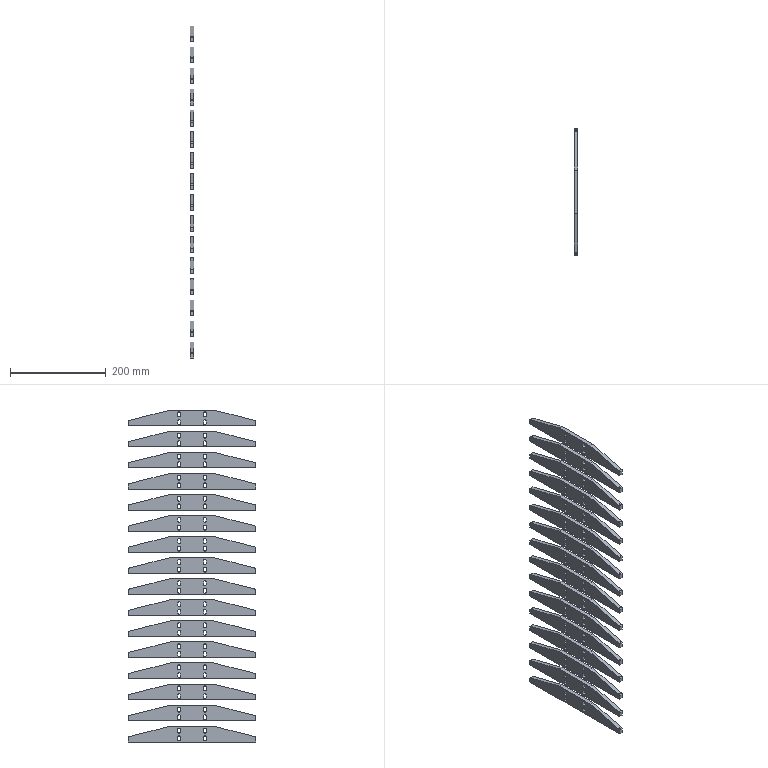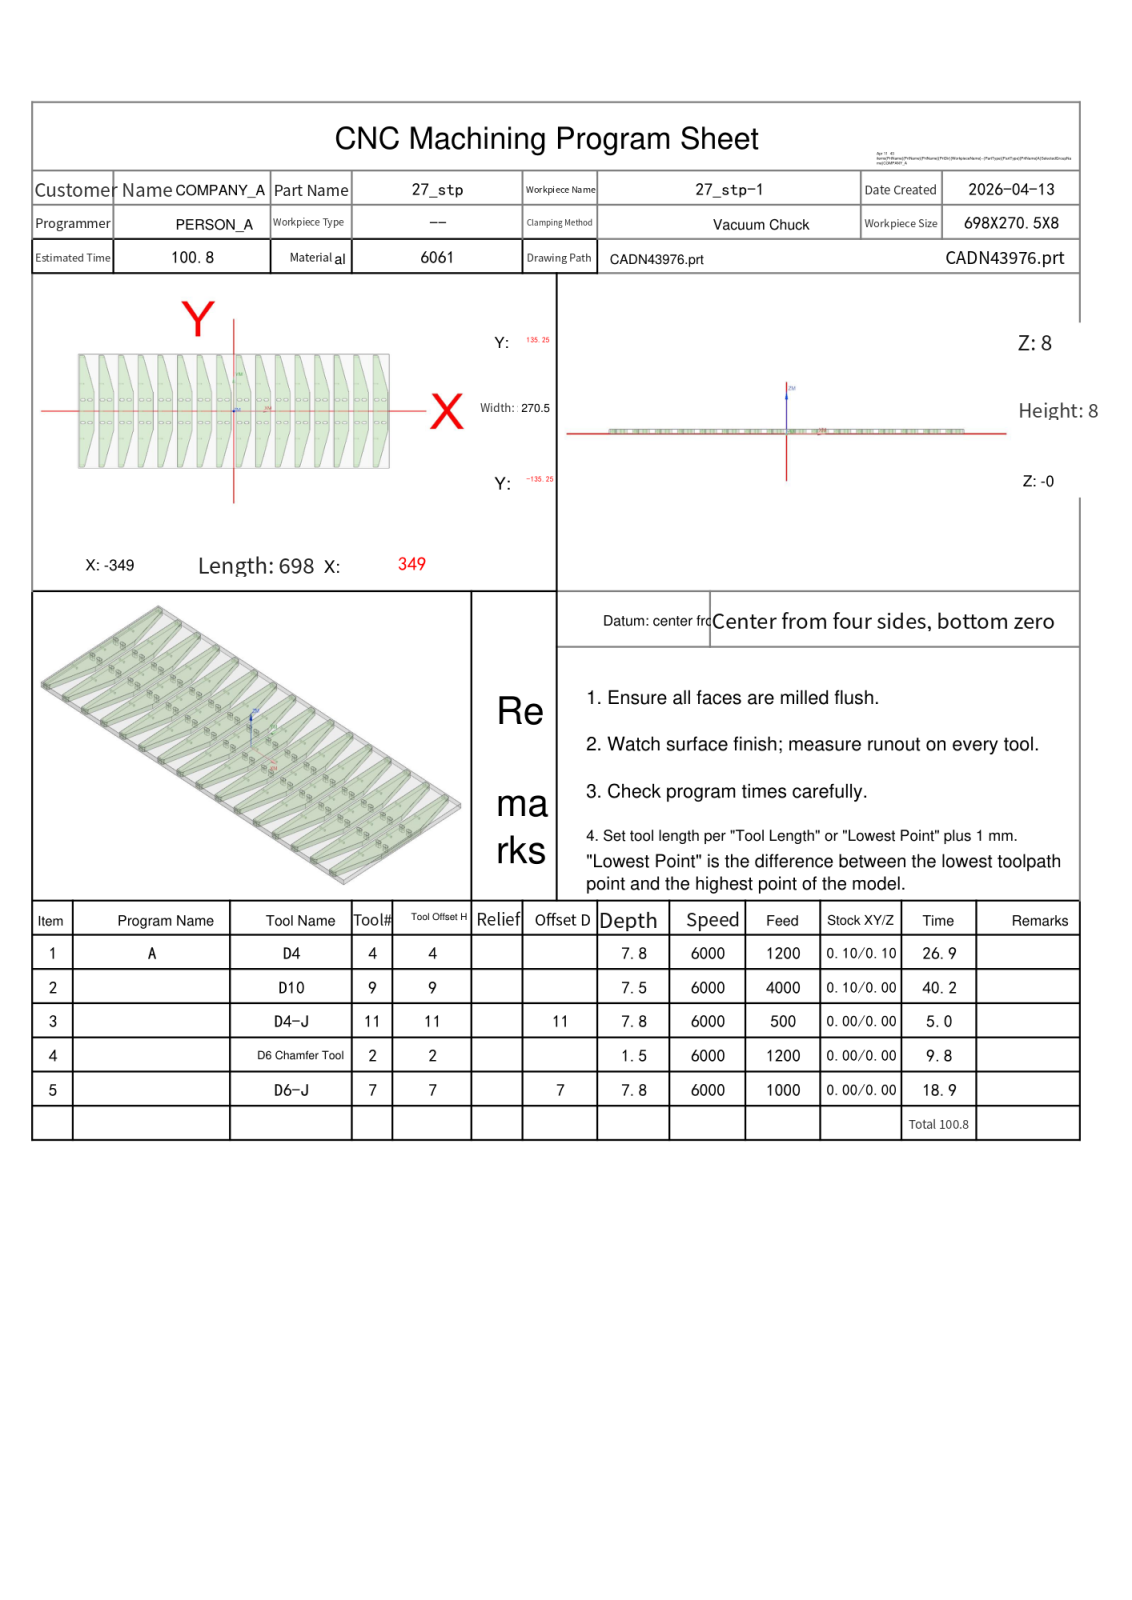NC program | NX | posted by the shop | part box 8 x 265.5 x 693 mm
Lines 14218 to 15115 of 21683:
N2 T09 M06
(D10  D=10. R=0. H=09 ce=0.10 di=0.00)
G00 G90 G54 X307.6 Y0.0 M03 S6000
G43 H09 Z28.
M08
Z8.5
G01 Y-45.801 Z8.461 F4000.
X285.864 Y-131.736 Z8.386
G02 X278.012 Y-137.85 Z8.377 I-7.853 J1.986
G01 X269.5 Z8.37
G02 X264.4 Y-132.75 Z8.363 I0.0 J5.1
G01 Y132.75 Z8.137
G02 X269.5 Y137.85 Z8.13 I5.1 J0.0
G01 X278.012 Z8.123
G02 X285.864 Y131.736 Z8.114 I0.0 J-8.1
G01 X307.6 Y45.801 Z8.039
Y-45.801 Z7.961
X285.864 Y-131.736 Z7.886
G02 X278.012 Y-137.85 Z7.877 I-7.853 J1.986
G01 X269.5 Z7.87
G02 X264.4 Y-132.75 Z7.863 I0.0 J5.1
G01 Y132.75 Z7.637
G02 X269.5 Y137.85 Z7.63 I5.1 J0.0
G01 X278.012 Z7.623
G02 X285.864 Y131.736 Z7.614 I0.0 J-8.1
G01 X307.6 Y45.801 Z7.539
Y-45.801 Z7.461
X285.864 Y-131.736 Z7.386
G02 X278.012 Y-137.85 Z7.377 I-7.853 J1.986
G01 X269.5 Z7.37
G02 X264.4 Y-132.75 Z7.363 I0.0 J5.1
G01 Y132.75 Z7.137
G02 X269.5 Y137.85 Z7.13 I5.1 J0.0
G01 X278.012 Z7.123
G02 X285.864 Y131.736 Z7.114 I0.0 J-8.1
G01 X307.6 Y45.801 Z7.039
Y-45.801 Z6.961
X285.864 Y-131.736 Z6.886
G02 X278.012 Y-137.85 Z6.877 I-7.853 J1.986
G01 X269.5 Z6.87
G02 X264.4 Y-132.75 Z6.863 I0.0 J5.1
G01 Y132.75 Z6.637
G02 X269.5 Y137.85 Z6.63 I5.1 J0.0
G01 X278.012 Z6.623
G02 X285.864 Y131.736 Z6.614 I0.0 J-8.1
G01 X307.6 Y45.801 Z6.539
Y-45.801 Z6.461
X285.864 Y-131.736 Z6.386
G02 X278.012 Y-137.85 Z6.377 I-7.853 J1.986
G01 X269.5 Z6.37
G02 X264.4 Y-132.75 Z6.363 I0.0 J5.1
G01 Y132.75 Z6.137
G02 X269.5 Y137.85 Z6.13 I5.1 J0.0
G01 X278.012 Z6.123
G02 X285.864 Y131.736 Z6.114 I0.0 J-8.1
G01 X307.6 Y45.801 Z6.039
Y-45.801 Z5.961
X285.864 Y-131.736 Z5.886
G02 X278.012 Y-137.85 Z5.877 I-7.853 J1.986
G01 X269.5 Z5.87
G02 X264.4 Y-132.75 Z5.863 I0.0 J5.1
G01 Y132.75 Z5.637
G02 X269.5 Y137.85 Z5.63 I5.1 J0.0
G01 X278.012 Z5.623
G02 X285.864 Y131.736 Z5.614 I0.0 J-8.1
G01 X307.6 Y45.801 Z5.539
Y-45.801 Z5.461
X285.864 Y-131.736 Z5.386
G02 X278.012 Y-137.85 Z5.377 I-7.853 J1.986
G01 X269.5 Z5.37
G02 X264.4 Y-132.75 Z5.363 I0.0 J5.1
G01 Y132.75 Z5.137
G02 X269.5 Y137.85 Z5.13 I5.1 J0.0
G01 X278.012 Z5.123
G02 X285.864 Y131.736 Z5.114 I0.0 J-8.1
G01 X307.6 Y45.801 Z5.039
Y-45.801 Z4.961
X285.864 Y-131.736 Z4.886
G02 X278.012 Y-137.85 Z4.877 I-7.853 J1.986
G01 X269.5 Z4.87
G02 X264.4 Y-132.75 Z4.863 I0.0 J5.1
G01 Y132.75 Z4.637
G02 X269.5 Y137.85 Z4.63 I5.1 J0.0
G01 X278.012 Z4.623
G02 X285.864 Y131.736 Z4.614 I0.0 J-8.1
G01 X307.6 Y45.801 Z4.539
Y-45.801 Z4.461
X285.864 Y-131.736 Z4.386
G02 X278.012 Y-137.85 Z4.377 I-7.853 J1.986
G01 X269.5 Z4.37
G02 X264.4 Y-132.75 Z4.363 I0.0 J5.1
G01 Y132.75 Z4.137
G02 X269.5 Y137.85 Z4.13 I5.1 J0.0
G01 X278.012 Z4.123
G02 X285.864 Y131.736 Z4.114 I0.0 J-8.1
G01 X307.6 Y45.801 Z4.039
Y-45.801 Z3.961
X285.864 Y-131.736 Z3.886
G02 X278.012 Y-137.85 Z3.877 I-7.853 J1.986
G01 X269.5 Z3.87
G02 X264.4 Y-132.75 Z3.863 I0.0 J5.1
G01 Y132.75 Z3.637
G02 X269.5 Y137.85 Z3.63 I5.1 J0.0
G01 X278.012 Z3.623
G02 X285.864 Y131.736 Z3.614 I0.0 J-8.1
G01 X307.6 Y45.801 Z3.539
Y-45.801 Z3.461
X285.864 Y-131.736 Z3.386
G02 X278.012 Y-137.85 Z3.377 I-7.853 J1.986
G01 X269.5 Z3.37
G02 X264.4 Y-132.75 Z3.363 I0.0 J5.1
G01 Y132.75 Z3.137
G02 X269.5 Y137.85 Z3.13 I5.1 J0.0
G01 X278.012 Z3.123
G02 X285.864 Y131.736 Z3.114 I0.0 J-8.1
G01 X307.6 Y45.801 Z3.039
Y-45.801 Z2.961
X285.864 Y-131.736 Z2.886
G02 X278.012 Y-137.85 Z2.877 I-7.853 J1.986
G01 X269.5 Z2.87
G02 X264.4 Y-132.75 Z2.863 I0.0 J5.1
G01 Y132.75 Z2.637
G02 X269.5 Y137.85 Z2.63 I5.1 J0.0
G01 X278.012 Z2.623
G02 X285.864 Y131.736 Z2.614 I0.0 J-8.1
G01 X307.6 Y45.801 Z2.539
Y-45.801 Z2.461
X285.864 Y-131.736 Z2.386
G02 X278.012 Y-137.85 Z2.377 I-7.853 J1.986
G01 X269.5 Z2.37
G02 X264.4 Y-132.75 Z2.363 I0.0 J5.1
G01 Y132.75 Z2.137
G02 X269.5 Y137.85 Z2.13 I5.1 J0.0
G01 X278.012 Z2.123
G02 X285.864 Y131.736 Z2.114 I0.0 J-8.1
G01 X307.6 Y45.801 Z2.039
Y-45.801 Z1.961
X285.864 Y-131.736 Z1.886
G02 X278.012 Y-137.85 Z1.877 I-7.853 J1.986
G01 X269.5 Z1.87
G02 X264.4 Y-132.75 Z1.863 I0.0 J5.1
G01 Y132.75 Z1.637
G02 X269.5 Y137.85 Z1.63 I5.1 J0.0
G01 X278.012 Z1.623
G02 X285.864 Y131.736 Z1.614 I0.0 J-8.1
G01 X307.6 Y45.801 Z1.539
Y-45.801 Z1.461
X285.864 Y-131.736 Z1.386
G02 X278.012 Y-137.85 Z1.377 I-7.853 J1.986
G01 X269.5 Z1.37
G02 X264.4 Y-132.75 Z1.363 I0.0 J5.1
G01 Y132.75 Z1.137
G02 X269.5 Y137.85 Z1.13 I5.1 J0.0
G01 X278.012 Z1.123
G02 X285.864 Y131.736 Z1.114 I0.0 J-8.1
G01 X307.6 Y45.801 Z1.039
Y-45.801 Z.961
X285.864 Y-131.736 Z.886
G02 X278.012 Y-137.85 Z.877 I-7.853 J1.986
G01 X269.5 Z.87
G02 X264.4 Y-132.75 Z.863 I0.0 J5.1
G01 Y132.75 Z.637
G02 X269.5 Y137.85 Z.63 I5.1 J0.0
G01 X278.012 Z.623
G02 X285.864 Y131.736 Z.614 I0.0 J-8.1
G01 X307.6 Y45.801 Z.539
Y0.0 Z.5
Y-45.801
X285.864 Y-131.736
G02 X278.012 Y-137.85 I-7.853 J1.986
G01 X269.5
G02 X264.4 Y-132.75 I0.0 J5.1
G01 Y132.75
G02 X269.5 Y137.85 I5.1 J0.0
G01 X278.012
G02 X285.864 Y131.736 I0.0 J-8.1
G01 X307.6 Y45.801
Y0.0
Y-.5
Z1.5
G00 Z28.
X351.6 Y0.0
Z8.5
G01 Y-45.801 Z8.461
X329.864 Y-131.736 Z8.386
G02 X322.012 Y-137.85 Z8.377 I-7.853 J1.986
G01 X313.5 Z8.37
G02 X308.4 Y-132.75 Z8.363 I0.0 J5.1
G01 Y132.75 Z8.137
G02 X313.5 Y137.85 Z8.13 I5.1 J0.0
G01 X322.012 Z8.123
G02 X329.864 Y131.736 Z8.114 I0.0 J-8.1
G01 X351.6 Y45.801 Z8.039
Y-45.801 Z7.961
X329.864 Y-131.736 Z7.886
G02 X322.012 Y-137.85 Z7.877 I-7.853 J1.986
G01 X313.5 Z7.87
G02 X308.4 Y-132.75 Z7.863 I0.0 J5.1
G01 Y132.75 Z7.637
G02 X313.5 Y137.85 Z7.63 I5.1 J0.0
G01 X322.012 Z7.623
G02 X329.864 Y131.736 Z7.614 I0.0 J-8.1
G01 X351.6 Y45.801 Z7.539
Y-45.801 Z7.461
X329.864 Y-131.736 Z7.386
G02 X322.012 Y-137.85 Z7.377 I-7.853 J1.986
G01 X313.5 Z7.37
G02 X308.4 Y-132.75 Z7.363 I0.0 J5.1
G01 Y132.75 Z7.137
G02 X313.5 Y137.85 Z7.13 I5.1 J0.0
G01 X322.012 Z7.123
G02 X329.864 Y131.736 Z7.114 I0.0 J-8.1
G01 X351.6 Y45.801 Z7.039
Y-45.801 Z6.961
X329.864 Y-131.736 Z6.886
G02 X322.012 Y-137.85 Z6.877 I-7.853 J1.986
G01 X313.5 Z6.87
G02 X308.4 Y-132.75 Z6.863 I0.0 J5.1
G01 Y132.75 Z6.637
G02 X313.5 Y137.85 Z6.63 I5.1 J0.0
G01 X322.012 Z6.623
G02 X329.864 Y131.736 Z6.614 I0.0 J-8.1
G01 X351.6 Y45.801 Z6.539
Y-45.801 Z6.461
X329.864 Y-131.736 Z6.386
G02 X322.012 Y-137.85 Z6.377 I-7.853 J1.986
G01 X313.5 Z6.37
G02 X308.4 Y-132.75 Z6.363 I0.0 J5.1
G01 Y132.75 Z6.137
G02 X313.5 Y137.85 Z6.13 I5.1 J0.0
G01 X322.012 Z6.123
G02 X329.864 Y131.736 Z6.114 I0.0 J-8.1
G01 X351.6 Y45.801 Z6.039
Y-45.801 Z5.961
X329.864 Y-131.736 Z5.886
G02 X322.012 Y-137.85 Z5.877 I-7.853 J1.986
G01 X313.5 Z5.87
G02 X308.4 Y-132.75 Z5.863 I0.0 J5.1
G01 Y132.75 Z5.637
G02 X313.5 Y137.85 Z5.63 I5.1 J0.0
G01 X322.012 Z5.623
G02 X329.864 Y131.736 Z5.614 I0.0 J-8.1
G01 X351.6 Y45.801 Z5.539
Y-45.801 Z5.461
X329.864 Y-131.736 Z5.386
G02 X322.012 Y-137.85 Z5.377 I-7.853 J1.986
G01 X313.5 Z5.37
G02 X308.4 Y-132.75 Z5.363 I0.0 J5.1
G01 Y132.75 Z5.137
G02 X313.5 Y137.85 Z5.13 I5.1 J0.0
G01 X322.012 Z5.123
G02 X329.864 Y131.736 Z5.114 I0.0 J-8.1
G01 X351.6 Y45.801 Z5.039
Y-45.801 Z4.961
X329.864 Y-131.736 Z4.886
G02 X322.012 Y-137.85 Z4.877 I-7.853 J1.986
G01 X313.5 Z4.87
G02 X308.4 Y-132.75 Z4.863 I0.0 J5.1
G01 Y132.75 Z4.637
G02 X313.5 Y137.85 Z4.63 I5.1 J0.0
G01 X322.012 Z4.623
G02 X329.864 Y131.736 Z4.614 I0.0 J-8.1
G01 X351.6 Y45.801 Z4.539
Y-45.801 Z4.461
X329.864 Y-131.736 Z4.386
G02 X322.012 Y-137.85 Z4.377 I-7.853 J1.986
G01 X313.5 Z4.37
G02 X308.4 Y-132.75 Z4.363 I0.0 J5.1
G01 Y132.75 Z4.137
G02 X313.5 Y137.85 Z4.13 I5.1 J0.0
G01 X322.012 Z4.123
G02 X329.864 Y131.736 Z4.114 I0.0 J-8.1
G01 X351.6 Y45.801 Z4.039
Y-45.801 Z3.961
X329.864 Y-131.736 Z3.886
G02 X322.012 Y-137.85 Z3.877 I-7.853 J1.986
G01 X313.5 Z3.87
G02 X308.4 Y-132.75 Z3.863 I0.0 J5.1
G01 Y132.75 Z3.637
G02 X313.5 Y137.85 Z3.63 I5.1 J0.0
G01 X322.012 Z3.623
G02 X329.864 Y131.736 Z3.614 I0.0 J-8.1
G01 X351.6 Y45.801 Z3.539
Y-45.801 Z3.461
X329.864 Y-131.736 Z3.386
G02 X322.012 Y-137.85 Z3.377 I-7.853 J1.986
G01 X313.5 Z3.37
G02 X308.4 Y-132.75 Z3.363 I0.0 J5.1
G01 Y132.75 Z3.137
G02 X313.5 Y137.85 Z3.13 I5.1 J0.0
G01 X322.012 Z3.123
G02 X329.864 Y131.736 Z3.114 I0.0 J-8.1
G01 X351.6 Y45.801 Z3.039
Y-45.801 Z2.961
X329.864 Y-131.736 Z2.886
G02 X322.012 Y-137.85 Z2.877 I-7.853 J1.986
G01 X313.5 Z2.87
G02 X308.4 Y-132.75 Z2.863 I0.0 J5.1
G01 Y132.75 Z2.637
G02 X313.5 Y137.85 Z2.63 I5.1 J0.0
G01 X322.012 Z2.623
G02 X329.864 Y131.736 Z2.614 I0.0 J-8.1
G01 X351.6 Y45.801 Z2.539
Y-45.801 Z2.461
X329.864 Y-131.736 Z2.386
G02 X322.012 Y-137.85 Z2.377 I-7.853 J1.986
G01 X313.5 Z2.37
G02 X308.4 Y-132.75 Z2.363 I0.0 J5.1
G01 Y132.75 Z2.137
G02 X313.5 Y137.85 Z2.13 I5.1 J0.0
G01 X322.012 Z2.123
G02 X329.864 Y131.736 Z2.114 I0.0 J-8.1
G01 X351.6 Y45.801 Z2.039
Y-45.801 Z1.961
X329.864 Y-131.736 Z1.886
G02 X322.012 Y-137.85 Z1.877 I-7.853 J1.986
G01 X313.5 Z1.87
G02 X308.4 Y-132.75 Z1.863 I0.0 J5.1
G01 Y132.75 Z1.637
G02 X313.5 Y137.85 Z1.63 I5.1 J0.0
G01 X322.012 Z1.623
G02 X329.864 Y131.736 Z1.614 I0.0 J-8.1
G01 X351.6 Y45.801 Z1.539
Y-45.801 Z1.461
X329.864 Y-131.736 Z1.386
G02 X322.012 Y-137.85 Z1.377 I-7.853 J1.986
G01 X313.5 Z1.37
G02 X308.4 Y-132.75 Z1.363 I0.0 J5.1
G01 Y132.75 Z1.137
G02 X313.5 Y137.85 Z1.13 I5.1 J0.0
G01 X322.012 Z1.123
G02 X329.864 Y131.736 Z1.114 I0.0 J-8.1
G01 X351.6 Y45.801 Z1.039
Y-45.801 Z.961
X329.864 Y-131.736 Z.886
G02 X322.012 Y-137.85 Z.877 I-7.853 J1.986
G01 X313.5 Z.87
G02 X308.4 Y-132.75 Z.863 I0.0 J5.1
G01 Y132.75 Z.637
G02 X313.5 Y137.85 Z.63 I5.1 J0.0
G01 X322.012 Z.623
G02 X329.864 Y131.736 Z.614 I0.0 J-8.1
G01 X351.6 Y45.801 Z.539
Y0.0 Z.5
Y-45.801
X329.864 Y-131.736
G02 X322.012 Y-137.85 I-7.853 J1.986
G01 X313.5
G02 X308.4 Y-132.75 I0.0 J5.1
G01 Y132.75
G02 X313.5 Y137.85 I5.1 J0.0
G01 X322.012
G02 X329.864 Y131.736 I0.0 J-8.1
G01 X351.6 Y45.801
Y0.0
Y-.5
Z1.5
G00 Z28.
X263.6 Y0.0
Z8.5
G01 Y-45.801 Z8.461
X241.864 Y-131.736 Z8.386
G02 X234.012 Y-137.85 Z8.377 I-7.853 J1.986
G01 X225.5 Z8.37
G02 X220.4 Y-132.75 Z8.363 I0.0 J5.1
G01 Y132.75 Z8.137
G02 X225.5 Y137.85 Z8.13 I5.1 J0.0
G01 X234.012 Z8.123
G02 X241.864 Y131.736 Z8.114 I0.0 J-8.1
G01 X263.6 Y45.801 Z8.039
Y-45.801 Z7.961
X241.864 Y-131.736 Z7.886
G02 X234.012 Y-137.85 Z7.877 I-7.853 J1.986
G01 X225.5 Z7.87
G02 X220.4 Y-132.75 Z7.863 I0.0 J5.1
G01 Y132.75 Z7.637
G02 X225.5 Y137.85 Z7.63 I5.1 J0.0
G01 X234.012 Z7.623
G02 X241.864 Y131.736 Z7.614 I0.0 J-8.1
G01 X263.6 Y45.801 Z7.539
Y-45.801 Z7.461
X241.864 Y-131.736 Z7.386
G02 X234.012 Y-137.85 Z7.377 I-7.853 J1.986
G01 X225.5 Z7.37
G02 X220.4 Y-132.75 Z7.363 I0.0 J5.1
G01 Y132.75 Z7.137
G02 X225.5 Y137.85 Z7.13 I5.1 J0.0
G01 X234.012 Z7.123
G02 X241.864 Y131.736 Z7.114 I0.0 J-8.1
G01 X263.6 Y45.801 Z7.039
Y-45.801 Z6.961
X241.864 Y-131.736 Z6.886
G02 X234.012 Y-137.85 Z6.877 I-7.853 J1.986
G01 X225.5 Z6.87
G02 X220.4 Y-132.75 Z6.863 I0.0 J5.1
G01 Y132.75 Z6.637
G02 X225.5 Y137.85 Z6.63 I5.1 J0.0
G01 X234.012 Z6.623
G02 X241.864 Y131.736 Z6.614 I0.0 J-8.1
G01 X263.6 Y45.801 Z6.539
Y-45.801 Z6.461
X241.864 Y-131.736 Z6.386
G02 X234.012 Y-137.85 Z6.377 I-7.853 J1.986
G01 X225.5 Z6.37
G02 X220.4 Y-132.75 Z6.363 I0.0 J5.1
G01 Y132.75 Z6.137
G02 X225.5 Y137.85 Z6.13 I5.1 J0.0
G01 X234.012 Z6.123
G02 X241.864 Y131.736 Z6.114 I0.0 J-8.1
G01 X263.6 Y45.801 Z6.039
Y-45.801 Z5.961
X241.864 Y-131.736 Z5.886
G02 X234.012 Y-137.85 Z5.877 I-7.853 J1.986
G01 X225.5 Z5.87
G02 X220.4 Y-132.75 Z5.863 I0.0 J5.1
G01 Y132.75 Z5.637
G02 X225.5 Y137.85 Z5.63 I5.1 J0.0
G01 X234.012 Z5.623
G02 X241.864 Y131.736 Z5.614 I0.0 J-8.1
G01 X263.6 Y45.801 Z5.539
Y-45.801 Z5.461
X241.864 Y-131.736 Z5.386
G02 X234.012 Y-137.85 Z5.377 I-7.853 J1.986
G01 X225.5 Z5.37
G02 X220.4 Y-132.75 Z5.363 I0.0 J5.1
G01 Y132.75 Z5.137
G02 X225.5 Y137.85 Z5.13 I5.1 J0.0
G01 X234.012 Z5.123
G02 X241.864 Y131.736 Z5.114 I0.0 J-8.1
G01 X263.6 Y45.801 Z5.039
Y-45.801 Z4.961
X241.864 Y-131.736 Z4.886
G02 X234.012 Y-137.85 Z4.877 I-7.853 J1.986
G01 X225.5 Z4.87
G02 X220.4 Y-132.75 Z4.863 I0.0 J5.1
G01 Y132.75 Z4.637
G02 X225.5 Y137.85 Z4.63 I5.1 J0.0
G01 X234.012 Z4.623
G02 X241.864 Y131.736 Z4.614 I0.0 J-8.1
G01 X263.6 Y45.801 Z4.539
Y-45.801 Z4.461
X241.864 Y-131.736 Z4.386
G02 X234.012 Y-137.85 Z4.377 I-7.853 J1.986
G01 X225.5 Z4.37
G02 X220.4 Y-132.75 Z4.363 I0.0 J5.1
G01 Y132.75 Z4.137
G02 X225.5 Y137.85 Z4.13 I5.1 J0.0
G01 X234.012 Z4.123
G02 X241.864 Y131.736 Z4.114 I0.0 J-8.1
G01 X263.6 Y45.801 Z4.039
Y-45.801 Z3.961
X241.864 Y-131.736 Z3.886
G02 X234.012 Y-137.85 Z3.877 I-7.853 J1.986
G01 X225.5 Z3.87
G02 X220.4 Y-132.75 Z3.863 I0.0 J5.1
G01 Y132.75 Z3.637
G02 X225.5 Y137.85 Z3.63 I5.1 J0.0
G01 X234.012 Z3.623
G02 X241.864 Y131.736 Z3.614 I0.0 J-8.1
G01 X263.6 Y45.801 Z3.539
Y-45.801 Z3.461
X241.864 Y-131.736 Z3.386
G02 X234.012 Y-137.85 Z3.377 I-7.853 J1.986
G01 X225.5 Z3.37
G02 X220.4 Y-132.75 Z3.363 I0.0 J5.1
G01 Y132.75 Z3.137
G02 X225.5 Y137.85 Z3.13 I5.1 J0.0
G01 X234.012 Z3.123
G02 X241.864 Y131.736 Z3.114 I0.0 J-8.1
G01 X263.6 Y45.801 Z3.039
Y-45.801 Z2.961
X241.864 Y-131.736 Z2.886
G02 X234.012 Y-137.85 Z2.877 I-7.853 J1.986
G01 X225.5 Z2.87
G02 X220.4 Y-132.75 Z2.863 I0.0 J5.1
G01 Y132.75 Z2.637
G02 X225.5 Y137.85 Z2.63 I5.1 J0.0
G01 X234.012 Z2.623
G02 X241.864 Y131.736 Z2.614 I0.0 J-8.1
G01 X263.6 Y45.801 Z2.539
Y-45.801 Z2.461
X241.864 Y-131.736 Z2.386
G02 X234.012 Y-137.85 Z2.377 I-7.853 J1.986
G01 X225.5 Z2.37
G02 X220.4 Y-132.75 Z2.363 I0.0 J5.1
G01 Y132.75 Z2.137
G02 X225.5 Y137.85 Z2.13 I5.1 J0.0
G01 X234.012 Z2.123
G02 X241.864 Y131.736 Z2.114 I0.0 J-8.1
G01 X263.6 Y45.801 Z2.039
Y-45.801 Z1.961
X241.864 Y-131.736 Z1.886
G02 X234.012 Y-137.85 Z1.877 I-7.853 J1.986
G01 X225.5 Z1.87
G02 X220.4 Y-132.75 Z1.863 I0.0 J5.1
G01 Y132.75 Z1.637
G02 X225.5 Y137.85 Z1.63 I5.1 J0.0
G01 X234.012 Z1.623
G02 X241.864 Y131.736 Z1.614 I0.0 J-8.1
G01 X263.6 Y45.801 Z1.539
Y-45.801 Z1.461
X241.864 Y-131.736 Z1.386
G02 X234.012 Y-137.85 Z1.377 I-7.853 J1.986
G01 X225.5 Z1.37
G02 X220.4 Y-132.75 Z1.363 I0.0 J5.1
G01 Y132.75 Z1.137
G02 X225.5 Y137.85 Z1.13 I5.1 J0.0
G01 X234.012 Z1.123
G02 X241.864 Y131.736 Z1.114 I0.0 J-8.1
G01 X263.6 Y45.801 Z1.039
Y-45.801 Z.961
X241.864 Y-131.736 Z.886
G02 X234.012 Y-137.85 Z.877 I-7.853 J1.986
G01 X225.5 Z.87
G02 X220.4 Y-132.75 Z.863 I0.0 J5.1
G01 Y132.75 Z.637
G02 X225.5 Y137.85 Z.63 I5.1 J0.0
G01 X234.012 Z.623
G02 X241.864 Y131.736 Z.614 I0.0 J-8.1
G01 X263.6 Y45.801 Z.539
Y0.0 Z.5
Y-45.801
X241.864 Y-131.736
G02 X234.012 Y-137.85 I-7.853 J1.986
G01 X225.5
G02 X220.4 Y-132.75 I0.0 J5.1
G01 Y132.75
G02 X225.5 Y137.85 I5.1 J0.0
G01 X234.012
G02 X241.864 Y131.736 I0.0 J-8.1
G01 X263.6 Y45.801
Y0.0
Y-.5
Z1.5
G00 Z28.
X219.6 Y0.0
Z8.5
G01 Y-45.801 Z8.461
X197.864 Y-131.736 Z8.386
G02 X190.012 Y-137.85 Z8.377 I-7.853 J1.986
G01 X181.5 Z8.37
G02 X176.4 Y-132.75 Z8.363 I0.0 J5.1
G01 Y132.75 Z8.137
G02 X181.5 Y137.85 Z8.13 I5.1 J0.0
G01 X190.012 Z8.123
G02 X197.864 Y131.736 Z8.114 I0.0 J-8.1
G01 X219.6 Y45.801 Z8.039
Y-45.801 Z7.961
X197.864 Y-131.736 Z7.886
G02 X190.012 Y-137.85 Z7.877 I-7.853 J1.986
G01 X181.5 Z7.87
G02 X176.4 Y-132.75 Z7.863 I0.0 J5.1
G01 Y132.75 Z7.637
G02 X181.5 Y137.85 Z7.63 I5.1 J0.0
G01 X190.012 Z7.623
G02 X197.864 Y131.736 Z7.614 I0.0 J-8.1
G01 X219.6 Y45.801 Z7.539
Y-45.801 Z7.461
X197.864 Y-131.736 Z7.386
G02 X190.012 Y-137.85 Z7.377 I-7.853 J1.986
G01 X181.5 Z7.37
G02 X176.4 Y-132.75 Z7.363 I0.0 J5.1
G01 Y132.75 Z7.137
G02 X181.5 Y137.85 Z7.13 I5.1 J0.0
G01 X190.012 Z7.123
G02 X197.864 Y131.736 Z7.114 I0.0 J-8.1
G01 X219.6 Y45.801 Z7.039
Y-45.801 Z6.961
X197.864 Y-131.736 Z6.886
G02 X190.012 Y-137.85 Z6.877 I-7.853 J1.986
G01 X181.5 Z6.87
G02 X176.4 Y-132.75 Z6.863 I0.0 J5.1
G01 Y132.75 Z6.637
G02 X181.5 Y137.85 Z6.63 I5.1 J0.0
G01 X190.012 Z6.623
G02 X197.864 Y131.736 Z6.614 I0.0 J-8.1
G01 X219.6 Y45.801 Z6.539
Y-45.801 Z6.461
X197.864 Y-131.736 Z6.386
G02 X190.012 Y-137.85 Z6.377 I-7.853 J1.986
G01 X181.5 Z6.37
G02 X176.4 Y-132.75 Z6.363 I0.0 J5.1
G01 Y132.75 Z6.137
G02 X181.5 Y137.85 Z6.13 I5.1 J0.0
G01 X190.012 Z6.123
G02 X197.864 Y131.736 Z6.114 I0.0 J-8.1
G01 X219.6 Y45.801 Z6.039
Y-45.801 Z5.961
X197.864 Y-131.736 Z5.886
G02 X190.012 Y-137.85 Z5.877 I-7.853 J1.986
G01 X181.5 Z5.87
G02 X176.4 Y-132.75 Z5.863 I0.0 J5.1
G01 Y132.75 Z5.637
G02 X181.5 Y137.85 Z5.63 I5.1 J0.0
G01 X190.012 Z5.623
G02 X197.864 Y131.736 Z5.614 I0.0 J-8.1
G01 X219.6 Y45.801 Z5.539
Y-45.801 Z5.461
X197.864 Y-131.736 Z5.386
G02 X190.012 Y-137.85 Z5.377 I-7.853 J1.986
G01 X181.5 Z5.37
G02 X176.4 Y-132.75 Z5.363 I0.0 J5.1
G01 Y132.75 Z5.137
G02 X181.5 Y137.85 Z5.13 I5.1 J0.0
G01 X190.012 Z5.123
G02 X197.864 Y131.736 Z5.114 I0.0 J-8.1
G01 X219.6 Y45.801 Z5.039
Y-45.801 Z4.961
X197.864 Y-131.736 Z4.886
G02 X190.012 Y-137.85 Z4.877 I-7.853 J1.986
G01 X181.5 Z4.87
G02 X176.4 Y-132.75 Z4.863 I0.0 J5.1
G01 Y132.75 Z4.637
G02 X181.5 Y137.85 Z4.63 I5.1 J0.0
G01 X190.012 Z4.623
G02 X197.864 Y131.736 Z4.614 I0.0 J-8.1
G01 X219.6 Y45.801 Z4.539
Y-45.801 Z4.461
X197.864 Y-131.736 Z4.386
G02 X190.012 Y-137.85 Z4.377 I-7.853 J1.986
G01 X181.5 Z4.37
G02 X176.4 Y-132.75 Z4.363 I0.0 J5.1
G01 Y132.75 Z4.137
G02 X181.5 Y137.85 Z4.13 I5.1 J0.0
G01 X190.012 Z4.123
G02 X197.864 Y131.736 Z4.114 I0.0 J-8.1
G01 X219.6 Y45.801 Z4.039
Y-45.801 Z3.961
X197.864 Y-131.736 Z3.886
G02 X190.012 Y-137.85 Z3.877 I-7.853 J1.986
G01 X181.5 Z3.87
G02 X176.4 Y-132.75 Z3.863 I0.0 J5.1
G01 Y132.75 Z3.637
G02 X181.5 Y137.85 Z3.63 I5.1 J0.0
G01 X190.012 Z3.623
G02 X197.864 Y131.736 Z3.614 I0.0 J-8.1
G01 X219.6 Y45.801 Z3.539
Y-45.801 Z3.461
X197.864 Y-131.736 Z3.386
G02 X190.012 Y-137.85 Z3.377 I-7.853 J1.986
G01 X181.5 Z3.37
G02 X176.4 Y-132.75 Z3.363 I0.0 J5.1
G01 Y132.75 Z3.137
G02 X181.5 Y137.85 Z3.13 I5.1 J0.0
G01 X190.012 Z3.123
G02 X197.864 Y131.736 Z3.114 I0.0 J-8.1
G01 X219.6 Y45.801 Z3.039
Y-45.801 Z2.961
X197.864 Y-131.736 Z2.886
G02 X190.012 Y-137.85 Z2.877 I-7.853 J1.986
G01 X181.5 Z2.87
G02 X176.4 Y-132.75 Z2.863 I0.0 J5.1
G01 Y132.75 Z2.637
G02 X181.5 Y137.85 Z2.63 I5.1 J0.0
G01 X190.012 Z2.623
G02 X197.864 Y131.736 Z2.614 I0.0 J-8.1
G01 X219.6 Y45.801 Z2.539
Y-45.801 Z2.461
X197.864 Y-131.736 Z2.386
G02 X190.012 Y-137.85 Z2.377 I-7.853 J1.986
G01 X181.5 Z2.37
G02 X176.4 Y-132.75 Z2.363 I0.0 J5.1
G01 Y132.75 Z2.137
G02 X181.5 Y137.85 Z2.13 I5.1 J0.0
G01 X190.012 Z2.123
G02 X197.864 Y131.736 Z2.114 I0.0 J-8.1
G01 X219.6 Y45.801 Z2.039
Y-45.801 Z1.961
X197.864 Y-131.736 Z1.886
G02 X190.012 Y-137.85 Z1.877 I-7.853 J1.986
G01 X181.5 Z1.87
G02 X176.4 Y-132.75 Z1.863 I0.0 J5.1
G01 Y132.75 Z1.637
G02 X181.5 Y137.85 Z1.63 I5.1 J0.0
G01 X190.012 Z1.623
G02 X197.864 Y131.736 Z1.614 I0.0 J-8.1
G01 X219.6 Y45.801 Z1.539
Y-45.801 Z1.461
X197.864 Y-131.736 Z1.386
G02 X190.012 Y-137.85 Z1.377 I-7.853 J1.986
G01 X181.5 Z1.37
G02 X176.4 Y-132.75 Z1.363 I0.0 J5.1
G01 Y132.75 Z1.137
G02 X181.5 Y137.85 Z1.13 I5.1 J0.0
G01 X190.012 Z1.123
G02 X197.864 Y131.736 Z1.114 I0.0 J-8.1
G01 X219.6 Y45.801 Z1.039
Y-45.801 Z.961
X197.864 Y-131.736 Z.886
G02 X190.012 Y-137.85 Z.877 I-7.853 J1.986
G01 X181.5 Z.87
G02 X176.4 Y-132.75 Z.863 I0.0 J5.1
G01 Y132.75 Z.637
G02 X181.5 Y137.85 Z.63 I5.1 J0.0
G01 X190.012 Z.623
G02 X197.864 Y131.736 Z.614 I0.0 J-8.1
G01 X219.6 Y45.801 Z.539
Y0.0 Z.5
Y-45.801
X197.864 Y-131.736
G02 X190.012 Y-137.85 I-7.853 J1.986
G01 X181.5
G02 X176.4 Y-132.75 I0.0 J5.1
G01 Y132.75
G02 X181.5 Y137.85 I5.1 J0.0
G01 X190.012
G02 X197.864 Y131.736 I0.0 J-8.1
G01 X219.6 Y45.801
Y0.0
Y-.5
Z1.5
G00 Z28.
X175.6 Y0.0
Z8.5
G01 Y-45.801 Z8.461
X153.864 Y-131.736 Z8.386
G02 X146.012 Y-137.85 Z8.377 I-7.853 J1.986
G01 X137.5 Z8.37
G02 X132.4 Y-132.75 Z8.363 I0.0 J5.1
G01 Y132.75 Z8.137
G02 X137.5 Y137.85 Z8.13 I5.1 J0.0
G01 X146.012 Z8.123
G02 X153.864 Y131.736 Z8.114 I0.0 J-8.1
G01 X175.6 Y45.801 Z8.039
Y-45.801 Z7.961
X153.864 Y-131.736 Z7.886
G02 X146.012 Y-137.85 Z7.877 I-7.853 J1.986
G01 X137.5 Z7.87
G02 X132.4 Y-132.75 Z7.863 I0.0 J5.1
G01 Y132.75 Z7.637
G02 X137.5 Y137.85 Z7.63 I5.1 J0.0
G01 X146.012 Z7.623
G02 X153.864 Y131.736 Z7.614 I0.0 J-8.1
G01 X175.6 Y45.801 Z7.539
Y-45.801 Z7.461
X153.864 Y-131.736 Z7.386
G02 X146.012 Y-137.85 Z7.377 I-7.853 J1.986
G01 X137.5 Z7.37
G02 X132.4 Y-132.75 Z7.363 I0.0 J5.1
G01 Y132.75 Z7.137
G02 X137.5 Y137.85 Z7.13 I5.1 J0.0
G01 X146.012 Z7.123
G02 X153.864 Y131.736 Z7.114 I0.0 J-8.1
G01 X175.6 Y45.801 Z7.039
Y-45.801 Z6.961
X153.864 Y-131.736 Z6.886
G02 X146.012 Y-137.85 Z6.877 I-7.853 J1.986
G01 X137.5 Z6.87
G02 X132.4 Y-132.75 Z6.863 I0.0 J5.1
G01 Y132.75 Z6.637
G02 X137.5 Y137.85 Z6.63 I5.1 J0.0
G01 X146.012 Z6.623
G02 X153.864 Y131.736 Z6.614 I0.0 J-8.1
G01 X175.6 Y45.801 Z6.539
Y-45.801 Z6.461
X153.864 Y-131.736 Z6.386
G02 X146.012 Y-137.85 Z6.377 I-7.853 J1.986
G01 X137.5 Z6.37
G02 X132.4 Y-132.75 Z6.363 I0.0 J5.1
G01 Y132.75 Z6.137
G02 X137.5 Y137.85 Z6.13 I5.1 J0.0
G01 X146.012 Z6.123
G02 X153.864 Y131.736 Z6.114 I0.0 J-8.1
G01 X175.6 Y45.801 Z6.039
Y-45.801 Z5.961
X153.864 Y-131.736 Z5.886
G02 X146.012 Y-137.85 Z5.877 I-7.853 J1.986
G01 X137.5 Z5.87
G02 X132.4 Y-132.75 Z5.863 I0.0 J5.1
G01 Y132.75 Z5.637
G02 X137.5 Y137.85 Z5.63 I5.1 J0.0
G01 X146.012 Z5.623
G02 X153.864 Y131.736 Z5.614 I0.0 J-8.1
G01 X175.6 Y45.801 Z5.539
Y-45.801 Z5.461
X153.864 Y-131.736 Z5.386
G02 X146.012 Y-137.85 Z5.377 I-7.853 J1.986
G01 X137.5 Z5.37
G02 X132.4 Y-132.75 Z5.363 I0.0 J5.1
G01 Y132.75 Z5.137
G02 X137.5 Y137.85 Z5.13 I5.1 J0.0
G01 X146.012 Z5.123
G02 X153.864 Y131.736 Z5.114 I0.0 J-8.1
G01 X175.6 Y45.801 Z5.039
Y-45.801 Z4.961
X153.864 Y-131.736 Z4.886
G02 X146.012 Y-137.85 Z4.877 I-7.853 J1.986
G01 X137.5 Z4.87
G02 X132.4 Y-132.75 Z4.863 I0.0 J5.1
G01 Y132.75 Z4.637
G02 X137.5 Y137.85 Z4.63 I5.1 J0.0
G01 X146.012 Z4.623
G02 X153.864 Y131.736 Z4.614 I0.0 J-8.1
G01 X175.6 Y45.801 Z4.539
Y-45.801 Z4.461
X153.864 Y-131.736 Z4.386
G02 X146.012 Y-137.85 Z4.377 I-7.853 J1.986
G01 X137.5 Z4.37
G02 X132.4 Y-132.75 Z4.363 I0.0 J5.1
G01 Y132.75 Z4.137
G02 X137.5 Y137.85 Z4.13 I5.1 J0.0
G01 X146.012 Z4.123
G02 X153.864 Y131.736 Z4.114 I0.0 J-8.1
G01 X175.6 Y45.801 Z4.039
Y-45.801 Z3.961
X153.864 Y-131.736 Z3.886
G02 X146.012 Y-137.85 Z3.877 I-7.853 J1.986
G01 X137.5 Z3.87
G02 X132.4 Y-132.75 Z3.863 I0.0 J5.1
G01 Y132.75 Z3.637
G02 X137.5 Y137.85 Z3.63 I5.1 J0.0
G01 X146.012 Z3.623
G02 X153.864 Y131.736 Z3.614 I0.0 J-8.1
G01 X175.6 Y45.801 Z3.539
Y-45.801 Z3.461
X153.864 Y-131.736 Z3.386
G02 X146.012 Y-137.85 Z3.377 I-7.853 J1.986
G01 X137.5 Z3.37
G02 X132.4 Y-132.75 Z3.363 I0.0 J5.1
G01 Y132.75 Z3.137
G02 X137.5 Y137.85 Z3.13 I5.1 J0.0
G01 X146.012 Z3.123
G02 X153.864 Y131.736 Z3.114 I0.0 J-8.1
G01 X175.6 Y45.801 Z3.039
Y-45.801 Z2.961
X153.864 Y-131.736 Z2.886
G02 X146.012 Y-137.85 Z2.877 I-7.853 J1.986
G01 X137.5 Z2.87
G02 X132.4 Y-132.75 Z2.863 I0.0 J5.1
G01 Y132.75 Z2.637
G02 X137.5 Y137.85 Z2.63 I5.1 J0.0
G01 X146.012 Z2.623
G02 X153.864 Y131.736 Z2.614 I0.0 J-8.1
G01 X175.6 Y45.801 Z2.539
Y-45.801 Z2.461
X153.864 Y-131.736 Z2.386
G02 X146.012 Y-137.85 Z2.377 I-7.853 J1.986
G01 X137.5 Z2.37
G02 X132.4 Y-132.75 Z2.363 I0.0 J5.1
G01 Y132.75 Z2.137
G02 X137.5 Y137.85 Z2.13 I5.1 J0.0
G01 X146.012 Z2.123
G02 X153.864 Y131.736 Z2.114 I0.0 J-8.1
G01 X175.6 Y45.801 Z2.039
Y-45.801 Z1.961
X153.864 Y-131.736 Z1.886
G02 X146.012 Y-137.85 Z1.877 I-7.853 J1.986
G01 X137.5 Z1.87
G02 X132.4 Y-132.75 Z1.863 I0.0 J5.1
G01 Y132.75 Z1.637
G02 X137.5 Y137.85 Z1.63 I5.1 J0.0
G01 X146.012 Z1.623
G02 X153.864 Y131.736 Z1.614 I0.0 J-8.1
G01 X175.6 Y45.801 Z1.539
Y-45.801 Z1.461
X153.864 Y-131.736 Z1.386
G02 X146.012 Y-137.85 Z1.377 I-7.853 J1.986
G01 X137.5 Z1.37
G02 X132.4 Y-132.75 Z1.363 I0.0 J5.1
G01 Y132.75 Z1.137
G02 X137.5 Y137.85 Z1.13 I5.1 J0.0
G01 X146.012 Z1.123
G02 X153.864 Y131.736 Z1.114 I0.0 J-8.1
G01 X175.6 Y45.801 Z1.039
Y-45.801 Z.961
X153.864 Y-131.736 Z.886
G02 X146.012 Y-137.85 Z.877 I-7.853 J1.986
G01 X137.5 Z.87
G02 X132.4 Y-132.75 Z.863 I0.0 J5.1
G01 Y132.75 Z.637
G02 X137.5 Y137.85 Z.63 I5.1 J0.0
G01 X146.012 Z.623
G02 X153.864 Y131.736 Z.614 I0.0 J-8.1
G01 X175.6 Y45.801 Z.539
Y0.0 Z.5
Y-45.801
X153.864 Y-131.736
G02 X146.012 Y-137.85 I-7.853 J1.986
G01 X137.5
G02 X132.4 Y-132.75 I0.0 J5.1
G01 Y132.75
G02 X137.5 Y137.85 I5.1 J0.0
G01 X146.012
G02 X153.864 Y131.736 I0.0 J-8.1
G01 X175.6 Y45.801
Y0.0
Y-.5
Z1.5
G00 Z28.
X131.6 Y0.0
Z8.5
G01 Y-45.801 Z8.461
X109.864 Y-131.736 Z8.386
G02 X102.012 Y-137.85 Z8.377 I-7.853 J1.986
G01 X93.5 Z8.37
G02 X88.4 Y-132.75 Z8.363 I0.0 J5.1
G01 Y132.75 Z8.137
G02 X93.5 Y137.85 Z8.13 I5.1 J0.0